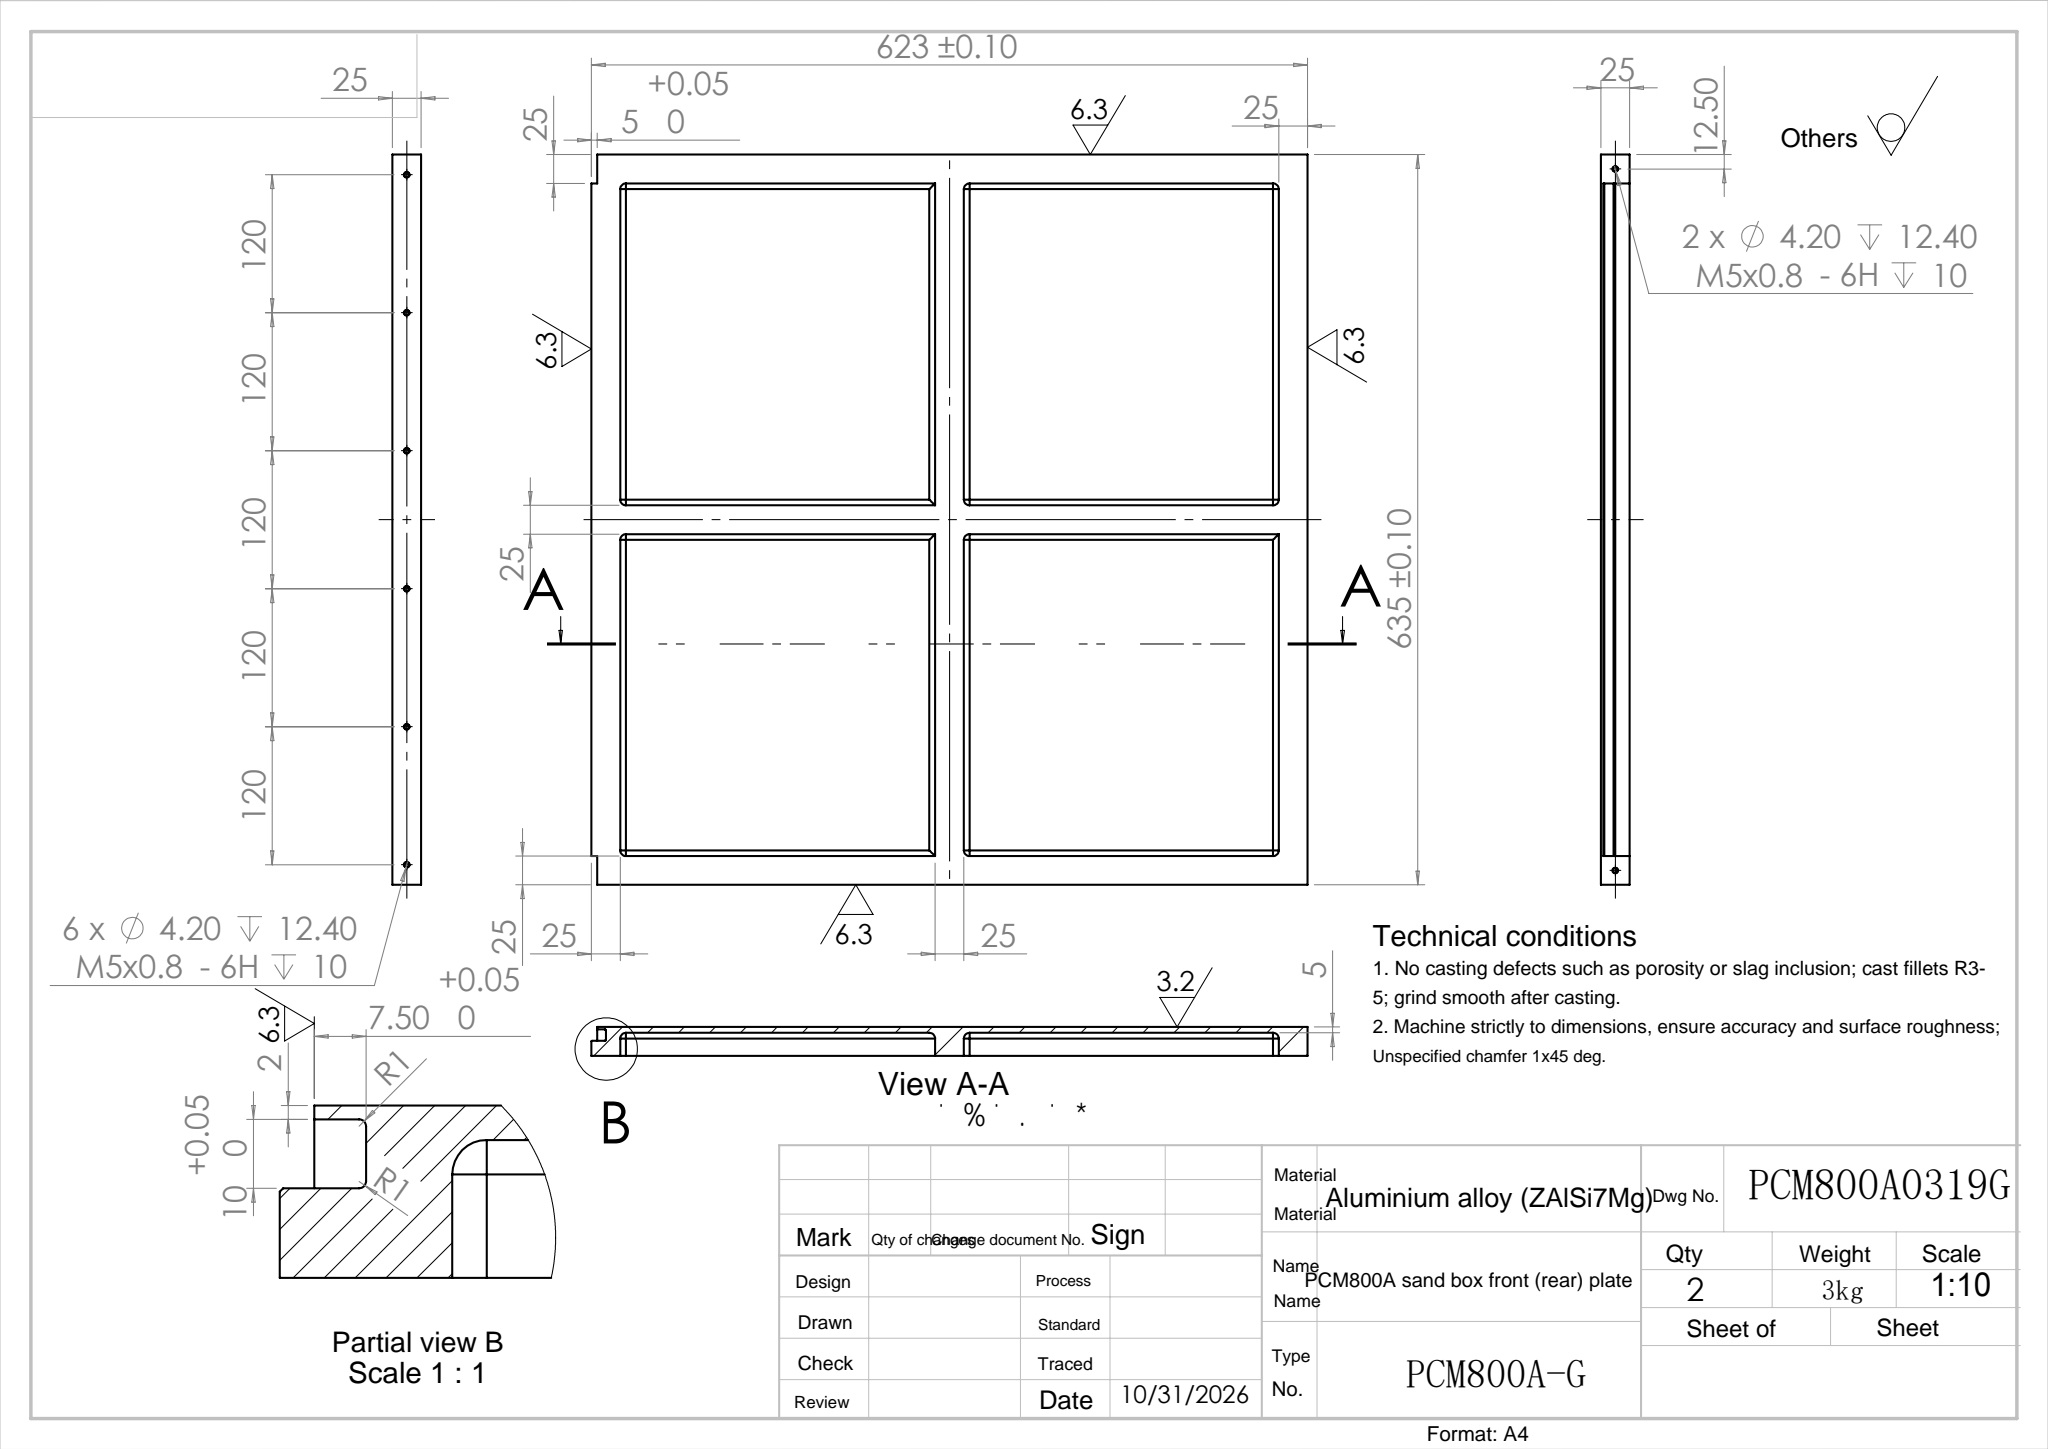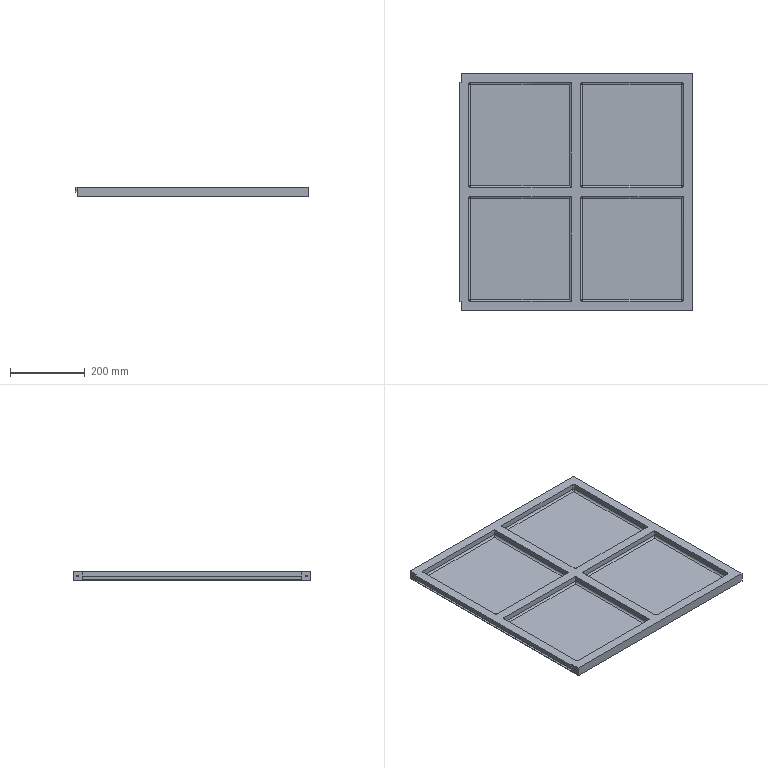Part | SolidWorks | features Boss 8, Cut 3, 3DProfileFeature 2, HoleWzd 2, Chamfer 1, Extrusion 1, Fillet 1 | 1 solid | 131 faces | box 623 x 635 x 25 mm | volume 3690263 mm3 | cylinder 61 | plane 43 | cone 16 | sphere 11 | commonest cylinder face diameters 10 x27 4.2 x16 5 x16 2 x2